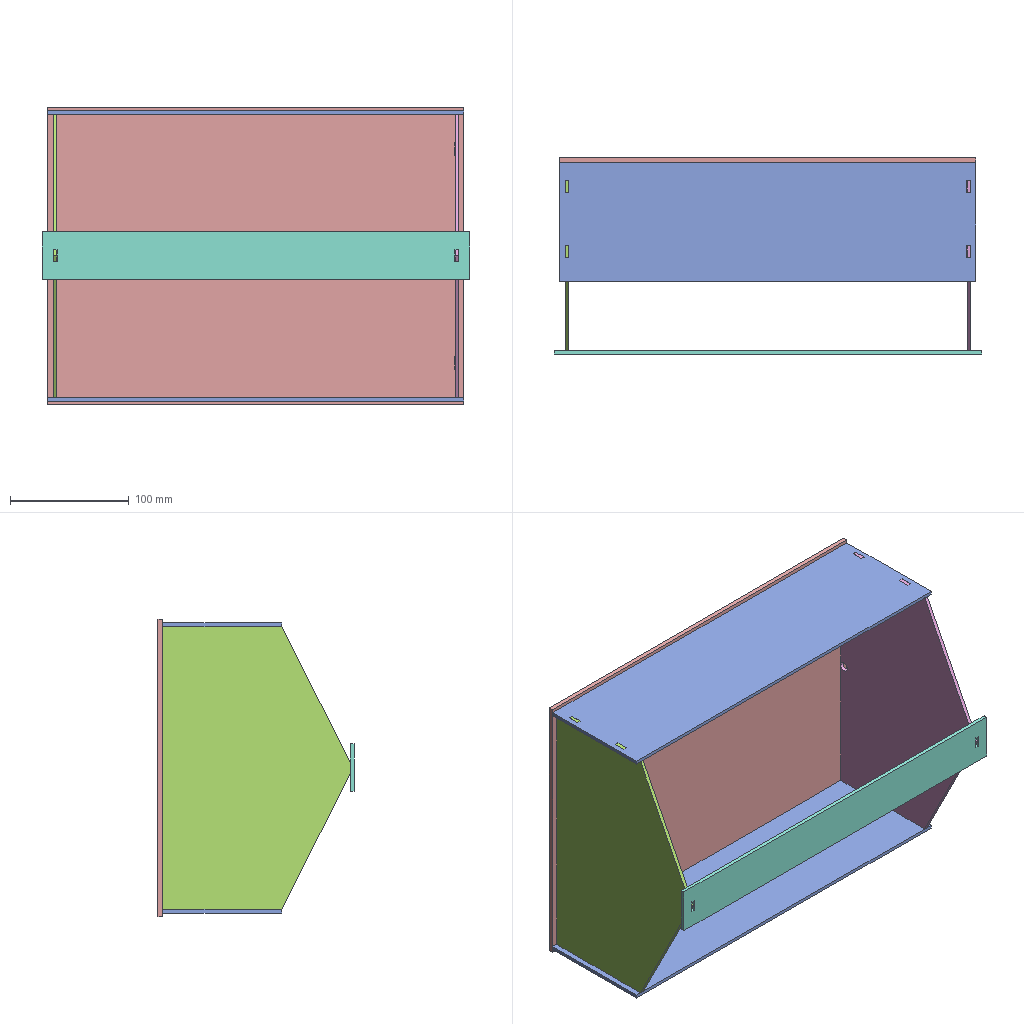Assembly | SolidWorks | 5 different items | 6 placed | box 360 x 165 x 250 mm
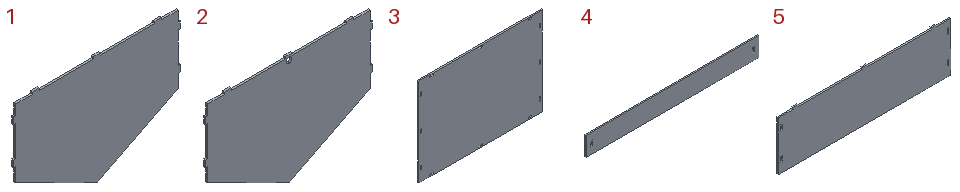Parts list (item | quantity | size | volume | features):
1 | x1 | 244 x 3 x 163 mm | 93450 mm3 | features Extrusion 1, ICE 1
2 | x1 | 244 x 3 x 163 mm | 93299 mm3 | features ICE 2, Extrusion 1
3 | x1 | 350 x 4 x 250 mm | 348433 mm3 | features ICE 2, Extrusion 1
4 | x1 | 360 x 3 x 40 mm | 43008 mm3 | features Extrusion 1, ICE 1
5 | x2 | 350 x 3 x 103 mm | 104878 mm3 | features ICE 2, Extrusion 1
Mates (type | each side: item.copy, entity, surface, feature):
Coincident | 3.1 face plane Boss-Extrude1 | 5.1 face plane Boss-Extrude1 | 2 times
Coincident | 3.1 face plane Boss-Extrude1 | 1.1 face plane Boss-Extrude1
Coincident | 5.1 face plane Boss-Extrude1 | 1.1 face plane Boss-Extrude1
DistanceDim | 5.1 face plane Cut-Extrude1 | 1.1 face plane Boss-Extrude1
Coincident | 3.1 face plane Boss-Extrude1 | 5.2 face plane Boss-Extrude1 | 3 times
Coincident | 5.2 face plane Boss-Extrude1 | 1.1 face plane Boss-Extrude1
DistanceDim | 5.2 face plane Cut-Extrude1 | 1.1 face plane Boss-Extrude1
DistanceDim | 5.2 face plane Boss-Extrude1 | 3.1 face plane Cut-Extrude2
Coincident | 3.1 face plane Boss-Extrude1 | 2.1 face plane Boss-Extrude1
Coincident | 5.1 face plane Boss-Extrude1 | 2.1 face plane Boss-Extrude1
DistanceDim | 5.1 face plane Cut-Extrude1 | 2.1 face plane Boss-Extrude1
Parallel | 3.1 face plane Boss-Extrude1 | 4.1 face plane Boss-Extrude1 | 2 times